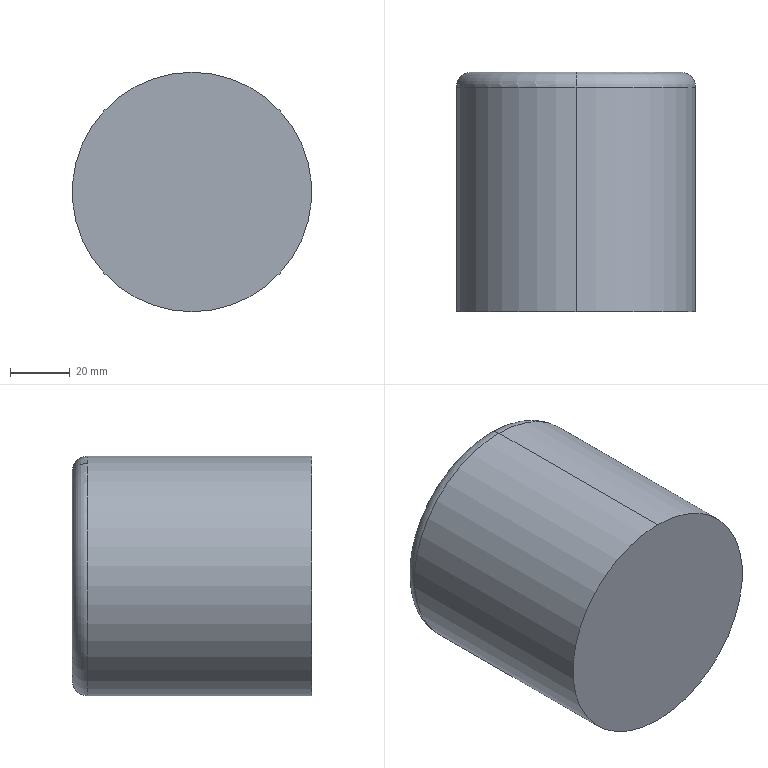Part | SolidWorks | features Extrusion 1, Fillet 1 | 1 solid | 6 faces | box 80 x 80 x 80 mm | volume 400813 mm3 | torus 2 | cylinder 2 | plane 2 | commonest cylinder face diameters 80 x2
STEP:
#1=CARTESIAN_POINT('',(0.,75.,-40.));
#2=VERTEX_POINT('',#1);
#3=CARTESIAN_POINT('',(0.,75.,40.));
#4=VERTEX_POINT('',#3);
#5=CARTESIAN_POINT('',(0.,75.,0.));
#6=DIRECTION('',(0.,-1.,0.));
#7=DIRECTION('',(0.,0.,1.));
#8=AXIS2_PLACEMENT_3D('',#5,#6,#7);
#9=CIRCLE('',#8,40.);
#10=EDGE_CURVE('',#2,#4,#9,.T.);
#11=ORIENTED_EDGE('',*,*,#10,.F.);
#12=CARTESIAN_POINT('',(0.,80.,-35.));
#13=VERTEX_POINT('',#12);
#14=CARTESIAN_POINT('',(0.,75.,-35.));
#15=DIRECTION('',(1.,0.,0.));
#16=DIRECTION('',(0.,0.,-1.));
#17=AXIS2_PLACEMENT_3D('',#14,#15,#16);
#18=CIRCLE('',#17,5.);
#19=EDGE_CURVE('',#2,#13,#18,.T.);
#20=ORIENTED_EDGE('',*,*,#19,.T.);
#21=CARTESIAN_POINT('',(0.,80.,35.));
#22=VERTEX_POINT('',#21);
#23=CARTESIAN_POINT('',(0.,80.,0.));
#24=DIRECTION('',(0.,1.,0.));
#25=DIRECTION('',(0.,0.,1.));
#26=AXIS2_PLACEMENT_3D('',#23,#24,#25);
#27=CIRCLE('',#26,35.);
#28=EDGE_CURVE('',#22,#13,#27,.T.);
#29=ORIENTED_EDGE('',*,*,#28,.F.);
#30=CARTESIAN_POINT('',(0.,75.,35.));
#31=DIRECTION('',(-1.,0.,0.));
#32=DIRECTION('',(0.,0.,1.));
#33=AXIS2_PLACEMENT_3D('',#30,#31,#32);
#34=CIRCLE('',#33,5.);
#35=EDGE_CURVE('',#4,#22,#34,.T.);
#36=ORIENTED_EDGE('',*,*,#35,.F.);
#37=EDGE_LOOP('',(#11,#20,#29,#36));
#38=FACE_OUTER_BOUND('',#37,.T.);
#39=CARTESIAN_POINT('',(0.,75.,0.));
#40=DIRECTION('',(0.,1.,0.));
#41=DIRECTION('',(0.,0.,1.));
#42=AXIS2_PLACEMENT_3D('',#39,#40,#41);
#43=TOROIDAL_SURFACE('',#42,35.,5.);
#44=ADVANCED_FACE('',(#38),#43,.T.);
#45=ORIENTED_EDGE('',*,*,#10,.T.);
#46=CARTESIAN_POINT('',(0.,0.,40.));
#47=VERTEX_POINT('',#46);
#48=CARTESIAN_POINT('',(0.,80.,40.));
#49=DIRECTION('',(0.,-1.,0.));
#50=VECTOR('',#49,1000.);
#51=LINE('',#48,#50);
#52=EDGE_CURVE('',#4,#47,#51,.T.);
#53=ORIENTED_EDGE('',*,*,#52,.T.);
#54=CARTESIAN_POINT('',(0.,0.,-40.));
#55=VERTEX_POINT('',#54);
#56=CARTESIAN_POINT('',(0.,0.,0.));
#57=DIRECTION('',(0.,1.,0.));
#58=DIRECTION('',(0.,0.,1.));
#59=AXIS2_PLACEMENT_3D('',#56,#57,#58);
#60=CIRCLE('',#59,40.);
#61=EDGE_CURVE('',#47,#55,#60,.T.);
#62=ORIENTED_EDGE('',*,*,#61,.T.);
#63=CARTESIAN_POINT('',(0.,80.,-40.));
#64=DIRECTION('',(0.,-1.,0.));
#65=VECTOR('',#64,1000.);
#66=LINE('',#63,#65);
#67=EDGE_CURVE('',#2,#55,#66,.T.);
#68=ORIENTED_EDGE('',*,*,#67,.F.);
#69=EDGE_LOOP('',(#45,#53,#62,#68));
#70=FACE_OUTER_BOUND('',#69,.T.);
#71=CARTESIAN_POINT('',(0.,80.,0.));
#72=DIRECTION('',(0.,-1.,0.));
#73=DIRECTION('',(0.,0.,-1.));
#74=AXIS2_PLACEMENT_3D('',#71,#72,#73);
#75=CYLINDRICAL_SURFACE('',#74,40.);
#76=ADVANCED_FACE('',(#70),#75,.T.);
#77=ORIENTED_EDGE('',*,*,#52,.F.);
#78=CARTESIAN_POINT('',(0.,75.,0.));
#79=DIRECTION('',(0.,-1.,0.));
#80=DIRECTION('',(0.,0.,1.));
#81=AXIS2_PLACEMENT_3D('',#78,#79,#80);
#82=CIRCLE('',#81,40.);
#83=EDGE_CURVE('',#4,#2,#82,.T.);
#84=ORIENTED_EDGE('',*,*,#83,.T.);
#85=ORIENTED_EDGE('',*,*,#67,.T.);
#86=CARTESIAN_POINT('',(0.,0.,0.));
#87=DIRECTION('',(0.,1.,0.));
#88=DIRECTION('',(0.,0.,1.));
#89=AXIS2_PLACEMENT_3D('',#86,#87,#88);
#90=CIRCLE('',#89,40.);
#91=EDGE_CURVE('',#55,#47,#90,.T.);
#92=ORIENTED_EDGE('',*,*,#91,.T.);
#93=EDGE_LOOP('',(#77,#84,#85,#92));
#94=FACE_OUTER_BOUND('',#93,.T.);
#95=CARTESIAN_POINT('',(0.,80.,0.));
#96=DIRECTION('',(0.,-1.,0.));
#97=DIRECTION('',(0.,0.,-1.));
#98=AXIS2_PLACEMENT_3D('',#95,#96,#97);
#99=CYLINDRICAL_SURFACE('',#98,40.);
#100=ADVANCED_FACE('',(#94),#99,.T.);
#101=ORIENTED_EDGE('',*,*,#28,.T.);
#102=CARTESIAN_POINT('',(0.,80.,0.));
#103=DIRECTION('',(0.,1.,0.));
#104=DIRECTION('',(0.,0.,1.));
#105=AXIS2_PLACEMENT_3D('',#102,#103,#104);
#106=CIRCLE('',#105,35.);
#107=EDGE_CURVE('',#13,#22,#106,.T.);
#108=ORIENTED_EDGE('',*,*,#107,.T.);
#109=EDGE_LOOP('',(#101,#108));
#110=FACE_OUTER_BOUND('',#109,.T.);
#111=CARTESIAN_POINT('',(0.,80.,0.));
#112=DIRECTION('',(0.,1.,0.));
#113=DIRECTION('',(0.,0.,1.));
#114=AXIS2_PLACEMENT_3D('',#111,#112,#113);
#115=PLANE('',#114);
#116=ADVANCED_FACE('',(#110),#115,.T.);
#117=ORIENTED_EDGE('',*,*,#91,.F.);
#118=ORIENTED_EDGE('',*,*,#61,.F.);
#119=EDGE_LOOP('',(#117,#118));
#120=FACE_OUTER_BOUND('',#119,.T.);
#121=CARTESIAN_POINT('',(0.,0.,0.));
#122=DIRECTION('',(0.,1.,0.));
#123=DIRECTION('',(0.,0.,1.));
#124=AXIS2_PLACEMENT_3D('',#121,#122,#123);
#125=PLANE('',#124);
#126=ADVANCED_FACE('',(#120),#125,.F.);
#127=ORIENTED_EDGE('',*,*,#19,.F.);
#128=ORIENTED_EDGE('',*,*,#83,.F.);
#129=ORIENTED_EDGE('',*,*,#35,.T.);
#130=ORIENTED_EDGE('',*,*,#107,.F.);
#131=EDGE_LOOP('',(#127,#128,#129,#130));
#132=FACE_OUTER_BOUND('',#131,.T.);
#133=CARTESIAN_POINT('',(0.,75.,0.));
#134=DIRECTION('',(0.,1.,0.));
#135=DIRECTION('',(0.,0.,1.));
#136=AXIS2_PLACEMENT_3D('',#133,#134,#135);
#137=TOROIDAL_SURFACE('',#136,35.,5.);
#138=ADVANCED_FACE('',(#132),#137,.T.);
#139=CLOSED_SHELL('',(#44,#76,#100,#116,#126,#138));
#140=MANIFOLD_SOLID_BREP('',#139);
#141=CARTESIAN_POINT('',(0.,0.,0.));
#142=DIRECTION('',(0.,0.,1.));
#143=DIRECTION('',(1.,0.,0.));
#144=AXIS2_PLACEMENT_3D('',#141,#142,#143);
#145=(LENGTH_UNIT()NAMED_UNIT(*)SI_UNIT(.MILLI.,.METRE.));
#146=UNCERTAINTY_MEASURE_WITH_UNIT(LENGTH_MEASURE(0.00001),#145,'','');
#147=(NAMED_UNIT(*)PLANE_ANGLE_UNIT()SI_UNIT($,.RADIAN.));
#148=(NAMED_UNIT(*)SI_UNIT($,.STERADIAN.)SOLID_ANGLE_UNIT());
#149=(GEOMETRIC_REPRESENTATION_CONTEXT(3)GLOBAL_UNCERTAINTY_ASSIGNED_CONTEXT((#146))GLOBAL_UNIT_ASSIGNED_CONTEXT((#145,#147,#148))REPRESENTATION_CONTEXT('',''));
#150=ADVANCED_BREP_SHAPE_REPRESENTATION('',(#140,#144),#149);